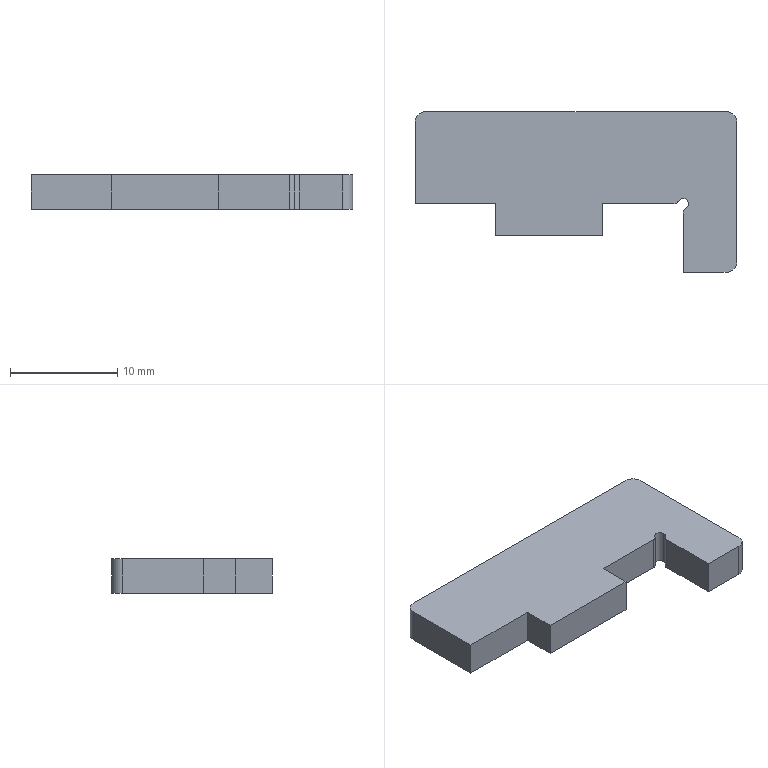Part | SolidWorks | features FlatPattern 1, SMBaseFlange 1, SheetMetal 1 | 1 solid | 19 faces | box 30 x 15 x 3.2 mm | volume 1020 mm3 | plane 12 | cylinder 7 | commonest cylinder face diameters 1 x4 2 x3
STEP:
#1=CARTESIAN_POINT('',(60.127,-203.35,-3.2));
#2=VERTEX_POINT('',#1);
#3=CARTESIAN_POINT('',(61.06,-203.6,-3.2));
#4=VERTEX_POINT('',#3);
#5=CARTESIAN_POINT('',(60.56,-203.6,-3.2));
#6=DIRECTION('',(0.,0.,-1.));
#7=DIRECTION('',(1.,0.,0.));
#8=AXIS2_PLACEMENT_3D('',#5,#6,#7);
#9=CIRCLE('',#8,0.5);
#10=EDGE_CURVE('',#2,#4,#9,.T.);
#11=ORIENTED_EDGE('',*,*,#10,.T.);
#12=CARTESIAN_POINT('',(61.06,-203.6,0.));
#13=VERTEX_POINT('',#12);
#14=CARTESIAN_POINT('',(61.06,-203.6,-3.2));
#15=DIRECTION('',(0.,0.,1.));
#16=VECTOR('',#15,1000.);
#17=LINE('',#14,#16);
#18=EDGE_CURVE('',#4,#13,#17,.T.);
#19=ORIENTED_EDGE('',*,*,#18,.T.);
#20=CARTESIAN_POINT('',(60.127,-203.35,0.));
#21=VERTEX_POINT('',#20);
#22=CARTESIAN_POINT('',(60.56,-203.6,0.));
#23=DIRECTION('',(0.,0.,-1.));
#24=DIRECTION('',(1.,0.,0.));
#25=AXIS2_PLACEMENT_3D('',#22,#23,#24);
#26=CIRCLE('',#25,0.5);
#27=EDGE_CURVE('',#21,#13,#26,.T.);
#28=ORIENTED_EDGE('',*,*,#27,.F.);
#29=CARTESIAN_POINT('',(60.127,-203.35,-3.2));
#30=DIRECTION('',(0.,0.,1.));
#31=VECTOR('',#30,1000.);
#32=LINE('',#29,#31);
#33=EDGE_CURVE('',#2,#21,#32,.T.);
#34=ORIENTED_EDGE('',*,*,#33,.F.);
#35=EDGE_LOOP('',(#11,#19,#28,#34));
#36=FACE_OUTER_BOUND('',#35,.T.);
#37=CARTESIAN_POINT('',(60.56,-203.6,-3.2));
#38=DIRECTION('',(0.,0.,1.));
#39=DIRECTION('',(1.,0.,0.));
#40=AXIS2_PLACEMENT_3D('',#37,#38,#39);
#41=CYLINDRICAL_SURFACE('',#40,0.5);
#42=ADVANCED_FACE('',(#36),#41,.F.);
#43=CARTESIAN_POINT('',(60.56,-204.466,0.));
#44=VERTEX_POINT('',#43);
#45=CARTESIAN_POINT('',(60.56,-210.,0.));
#46=VERTEX_POINT('',#45);
#47=CARTESIAN_POINT('',(60.56,-204.466,0.));
#48=DIRECTION('',(0.,-1.,0.));
#49=VECTOR('',#48,1000.);
#50=LINE('',#47,#49);
#51=EDGE_CURVE('',#44,#46,#50,.T.);
#52=ORIENTED_EDGE('',*,*,#51,.F.);
#53=CARTESIAN_POINT('',(60.56,-204.466,-3.2));
#54=VERTEX_POINT('',#53);
#55=CARTESIAN_POINT('',(60.56,-204.466,-3.2));
#56=DIRECTION('',(0.,0.,1.));
#57=VECTOR('',#56,1000.);
#58=LINE('',#55,#57);
#59=EDGE_CURVE('',#54,#44,#58,.T.);
#60=ORIENTED_EDGE('',*,*,#59,.F.);
#61=CARTESIAN_POINT('',(60.56,-210.,-3.2));
#62=VERTEX_POINT('',#61);
#63=CARTESIAN_POINT('',(60.56,-204.466,-3.2));
#64=DIRECTION('',(0.,-1.,0.));
#65=VECTOR('',#64,1000.);
#66=LINE('',#63,#65);
#67=EDGE_CURVE('',#54,#62,#66,.T.);
#68=ORIENTED_EDGE('',*,*,#67,.T.);
#69=CARTESIAN_POINT('',(60.56,-210.,-3.2));
#70=DIRECTION('',(0.,0.,1.));
#71=VECTOR('',#70,1000.);
#72=LINE('',#69,#71);
#73=EDGE_CURVE('',#62,#46,#72,.T.);
#74=ORIENTED_EDGE('',*,*,#73,.T.);
#75=EDGE_LOOP('',(#52,#60,#68,#74));
#76=FACE_OUTER_BOUND('',#75,.T.);
#77=CARTESIAN_POINT('',(60.56,-204.466,-3.2));
#78=DIRECTION('',(-1.,0.,0.));
#79=DIRECTION('',(0.,-1.,0.));
#80=AXIS2_PLACEMENT_3D('',#77,#78,#79);
#81=PLANE('',#80);
#82=ADVANCED_FACE('',(#76),#81,.T.);
#83=CARTESIAN_POINT('',(60.81,-204.033,0.));
#84=VERTEX_POINT('',#83);
#85=CARTESIAN_POINT('',(61.06,-204.466,0.));
#86=DIRECTION('',(0.,0.,1.));
#87=DIRECTION('',(1.,0.,0.));
#88=AXIS2_PLACEMENT_3D('',#85,#86,#87);
#89=CIRCLE('',#88,0.5);
#90=EDGE_CURVE('',#84,#44,#89,.T.);
#91=ORIENTED_EDGE('',*,*,#90,.F.);
#92=CARTESIAN_POINT('',(60.81,-204.033,-3.2));
#93=VERTEX_POINT('',#92);
#94=CARTESIAN_POINT('',(60.81,-204.033,-3.2));
#95=DIRECTION('',(0.,0.,1.));
#96=VECTOR('',#95,1000.);
#97=LINE('',#94,#96);
#98=EDGE_CURVE('',#93,#84,#97,.T.);
#99=ORIENTED_EDGE('',*,*,#98,.F.);
#100=CARTESIAN_POINT('',(61.06,-204.466,-3.2));
#101=DIRECTION('',(0.,0.,1.));
#102=DIRECTION('',(1.,0.,0.));
#103=AXIS2_PLACEMENT_3D('',#100,#101,#102);
#104=CIRCLE('',#103,0.5);
#105=EDGE_CURVE('',#93,#54,#104,.T.);
#106=ORIENTED_EDGE('',*,*,#105,.T.);
#107=ORIENTED_EDGE('',*,*,#59,.T.);
#108=EDGE_LOOP('',(#91,#99,#106,#107));
#109=FACE_OUTER_BOUND('',#108,.T.);
#110=CARTESIAN_POINT('',(61.06,-204.466,-3.2));
#111=DIRECTION('',(0.,0.,1.));
#112=DIRECTION('',(1.,0.,0.));
#113=AXIS2_PLACEMENT_3D('',#110,#111,#112);
#114=CYLINDRICAL_SURFACE('',#113,0.5);
#115=ADVANCED_FACE('',(#109),#114,.T.);
#116=ORIENTED_EDGE('',*,*,#18,.F.);
#117=CARTESIAN_POINT('',(60.56,-203.6,-3.2));
#118=DIRECTION('',(0.,0.,-1.));
#119=DIRECTION('',(1.,0.,0.));
#120=AXIS2_PLACEMENT_3D('',#117,#118,#119);
#121=CIRCLE('',#120,0.5);
#122=EDGE_CURVE('',#4,#93,#121,.T.);
#123=ORIENTED_EDGE('',*,*,#122,.T.);
#124=ORIENTED_EDGE('',*,*,#98,.T.);
#125=CARTESIAN_POINT('',(60.56,-203.6,0.));
#126=DIRECTION('',(0.,0.,-1.));
#127=DIRECTION('',(1.,0.,0.));
#128=AXIS2_PLACEMENT_3D('',#125,#126,#127);
#129=CIRCLE('',#128,0.5);
#130=EDGE_CURVE('',#13,#84,#129,.T.);
#131=ORIENTED_EDGE('',*,*,#130,.F.);
#132=EDGE_LOOP('',(#116,#123,#124,#131));
#133=FACE_OUTER_BOUND('',#132,.T.);
#134=CARTESIAN_POINT('',(60.56,-203.6,-3.2));
#135=DIRECTION('',(0.,0.,1.));
#136=DIRECTION('',(1.,0.,0.));
#137=AXIS2_PLACEMENT_3D('',#134,#135,#136);
#138=CYLINDRICAL_SURFACE('',#137,0.5);
#139=ADVANCED_FACE('',(#133),#138,.F.);
#140=CARTESIAN_POINT('',(59.694,-203.6,0.));
#141=VERTEX_POINT('',#140);
#142=CARTESIAN_POINT('',(59.694,-203.1,0.));
#143=DIRECTION('',(0.,0.,1.));
#144=DIRECTION('',(-1.,0.,0.));
#145=AXIS2_PLACEMENT_3D('',#142,#143,#144);
#146=CIRCLE('',#145,0.5);
#147=EDGE_CURVE('',#141,#21,#146,.T.);
#148=ORIENTED_EDGE('',*,*,#147,.F.);
#149=CARTESIAN_POINT('',(59.694,-203.6,-3.2));
#150=VERTEX_POINT('',#149);
#151=CARTESIAN_POINT('',(59.694,-203.6,-3.2));
#152=DIRECTION('',(0.,0.,1.));
#153=VECTOR('',#152,1000.);
#154=LINE('',#151,#153);
#155=EDGE_CURVE('',#150,#141,#154,.T.);
#156=ORIENTED_EDGE('',*,*,#155,.F.);
#157=CARTESIAN_POINT('',(59.694,-203.1,-3.2));
#158=DIRECTION('',(0.,0.,1.));
#159=DIRECTION('',(-1.,0.,0.));
#160=AXIS2_PLACEMENT_3D('',#157,#158,#159);
#161=CIRCLE('',#160,0.5);
#162=EDGE_CURVE('',#150,#2,#161,.T.);
#163=ORIENTED_EDGE('',*,*,#162,.T.);
#164=ORIENTED_EDGE('',*,*,#33,.T.);
#165=EDGE_LOOP('',(#148,#156,#163,#164));
#166=FACE_OUTER_BOUND('',#165,.T.);
#167=CARTESIAN_POINT('',(59.694,-203.1,-3.2));
#168=DIRECTION('',(0.,0.,1.));
#169=DIRECTION('',(1.,0.,0.));
#170=AXIS2_PLACEMENT_3D('',#167,#168,#169);
#171=CYLINDRICAL_SURFACE('',#170,0.5);
#172=ADVANCED_FACE('',(#166),#171,.T.);
#173=CARTESIAN_POINT('',(53.06,-203.6,0.));
#174=VERTEX_POINT('',#173);
#175=CARTESIAN_POINT('',(53.06,-203.6,0.));
#176=DIRECTION('',(1.,0.,0.));
#177=VECTOR('',#176,1000.);
#178=LINE('',#175,#177);
#179=EDGE_CURVE('',#174,#141,#178,.T.);
#180=ORIENTED_EDGE('',*,*,#179,.F.);
#181=CARTESIAN_POINT('',(53.06,-203.6,-3.2));
#182=VERTEX_POINT('',#181);
#183=CARTESIAN_POINT('',(53.06,-203.6,-3.2));
#184=DIRECTION('',(0.,0.,1.));
#185=VECTOR('',#184,1000.);
#186=LINE('',#183,#185);
#187=EDGE_CURVE('',#182,#174,#186,.T.);
#188=ORIENTED_EDGE('',*,*,#187,.F.);
#189=CARTESIAN_POINT('',(53.06,-203.6,-3.2));
#190=DIRECTION('',(1.,0.,0.));
#191=VECTOR('',#190,1000.);
#192=LINE('',#189,#191);
#193=EDGE_CURVE('',#182,#150,#192,.T.);
#194=ORIENTED_EDGE('',*,*,#193,.T.);
#195=ORIENTED_EDGE('',*,*,#155,.T.);
#196=EDGE_LOOP('',(#180,#188,#194,#195));
#197=FACE_OUTER_BOUND('',#196,.T.);
#198=CARTESIAN_POINT('',(53.06,-203.6,-3.2));
#199=DIRECTION('',(0.,-1.,0.));
#200=DIRECTION('',(0.,0.,-1.));
#201=AXIS2_PLACEMENT_3D('',#198,#199,#200);
#202=PLANE('',#201);
#203=ADVANCED_FACE('',(#197),#202,.T.);
#204=CARTESIAN_POINT('',(53.06,-206.6,0.));
#205=VERTEX_POINT('',#204);
#206=CARTESIAN_POINT('',(53.06,-206.6,0.));
#207=DIRECTION('',(0.,1.,0.));
#208=VECTOR('',#207,1000.);
#209=LINE('',#206,#208);
#210=EDGE_CURVE('',#205,#174,#209,.T.);
#211=ORIENTED_EDGE('',*,*,#210,.F.);
#212=CARTESIAN_POINT('',(53.06,-206.6,-3.2));
#213=VERTEX_POINT('',#212);
#214=CARTESIAN_POINT('',(53.06,-206.6,-3.2));
#215=DIRECTION('',(0.,0.,1.));
#216=VECTOR('',#215,1000.);
#217=LINE('',#214,#216);
#218=EDGE_CURVE('',#213,#205,#217,.T.);
#219=ORIENTED_EDGE('',*,*,#218,.F.);
#220=CARTESIAN_POINT('',(53.06,-206.6,-3.2));
#221=DIRECTION('',(0.,1.,0.));
#222=VECTOR('',#221,1000.);
#223=LINE('',#220,#222);
#224=EDGE_CURVE('',#213,#182,#223,.T.);
#225=ORIENTED_EDGE('',*,*,#224,.T.);
#226=ORIENTED_EDGE('',*,*,#187,.T.);
#227=EDGE_LOOP('',(#211,#219,#225,#226));
#228=FACE_OUTER_BOUND('',#227,.T.);
#229=CARTESIAN_POINT('',(53.06,-206.6,-3.2));
#230=DIRECTION('',(1.,0.,0.));
#231=DIRECTION('',(0.,0.,-1.));
#232=AXIS2_PLACEMENT_3D('',#229,#230,#231);
#233=PLANE('',#232);
#234=ADVANCED_FACE('',(#228),#233,.T.);
#235=CARTESIAN_POINT('',(43.06,-206.6,0.));
#236=VERTEX_POINT('',#235);
#237=CARTESIAN_POINT('',(43.06,-206.6,0.));
#238=DIRECTION('',(1.,0.,0.));
#239=VECTOR('',#238,1000.);
#240=LINE('',#237,#239);
#241=EDGE_CURVE('',#236,#205,#240,.T.);
#242=ORIENTED_EDGE('',*,*,#241,.F.);
#243=CARTESIAN_POINT('',(43.06,-206.6,-3.2));
#244=VERTEX_POINT('',#243);
#245=CARTESIAN_POINT('',(43.06,-206.6,-3.2));
#246=DIRECTION('',(0.,0.,1.));
#247=VECTOR('',#246,1000.);
#248=LINE('',#245,#247);
#249=EDGE_CURVE('',#244,#236,#248,.T.);
#250=ORIENTED_EDGE('',*,*,#249,.F.);
#251=CARTESIAN_POINT('',(43.06,-206.6,-3.2));
#252=DIRECTION('',(1.,0.,0.));
#253=VECTOR('',#252,1000.);
#254=LINE('',#251,#253);
#255=EDGE_CURVE('',#244,#213,#254,.T.);
#256=ORIENTED_EDGE('',*,*,#255,.T.);
#257=ORIENTED_EDGE('',*,*,#218,.T.);
#258=EDGE_LOOP('',(#242,#250,#256,#257));
#259=FACE_OUTER_BOUND('',#258,.T.);
#260=CARTESIAN_POINT('',(43.06,-206.6,-3.2));
#261=DIRECTION('',(0.,-1.,0.));
#262=DIRECTION('',(0.,0.,-1.));
#263=AXIS2_PLACEMENT_3D('',#260,#261,#262);
#264=PLANE('',#263);
#265=ADVANCED_FACE('',(#259),#264,.T.);
#266=CARTESIAN_POINT('',(43.06,-203.6,0.));
#267=VERTEX_POINT('',#266);
#268=CARTESIAN_POINT('',(43.06,-203.6,0.));
#269=DIRECTION('',(0.,-1.,0.));
#270=VECTOR('',#269,1000.);
#271=LINE('',#268,#270);
#272=EDGE_CURVE('',#267,#236,#271,.T.);
#273=ORIENTED_EDGE('',*,*,#272,.F.);
#274=CARTESIAN_POINT('',(43.06,-203.6,-3.2));
#275=VERTEX_POINT('',#274);
#276=CARTESIAN_POINT('',(43.06,-203.6,-3.2));
#277=DIRECTION('',(0.,0.,1.));
#278=VECTOR('',#277,1000.);
#279=LINE('',#276,#278);
#280=EDGE_CURVE('',#275,#267,#279,.T.);
#281=ORIENTED_EDGE('',*,*,#280,.F.);
#282=CARTESIAN_POINT('',(43.06,-203.6,-3.2));
#283=DIRECTION('',(0.,-1.,0.));
#284=VECTOR('',#283,1000.);
#285=LINE('',#282,#284);
#286=EDGE_CURVE('',#275,#244,#285,.T.);
#287=ORIENTED_EDGE('',*,*,#286,.T.);
#288=ORIENTED_EDGE('',*,*,#249,.T.);
#289=EDGE_LOOP('',(#273,#281,#287,#288));
#290=FACE_OUTER_BOUND('',#289,.T.);
#291=CARTESIAN_POINT('',(43.06,-203.6,-3.2));
#292=DIRECTION('',(-1.,0.,0.));
#293=DIRECTION('',(0.,0.,1.));
#294=AXIS2_PLACEMENT_3D('',#291,#292,#293);
#295=PLANE('',#294);
#296=ADVANCED_FACE('',(#290),#295,.T.);
#297=CARTESIAN_POINT('',(35.56,-203.6,0.));
#298=VERTEX_POINT('',#297);
#299=CARTESIAN_POINT('',(35.56,-203.6,0.));
#300=DIRECTION('',(1.,0.,0.));
#301=VECTOR('',#300,1000.);
#302=LINE('',#299,#301);
#303=EDGE_CURVE('',#298,#267,#302,.T.);
#304=ORIENTED_EDGE('',*,*,#303,.F.);
#305=CARTESIAN_POINT('',(35.56,-203.6,-3.2));
#306=VERTEX_POINT('',#305);
#307=CARTESIAN_POINT('',(35.56,-203.6,-3.2));
#308=DIRECTION('',(0.,0.,1.));
#309=VECTOR('',#308,1000.);
#310=LINE('',#307,#309);
#311=EDGE_CURVE('',#306,#298,#310,.T.);
#312=ORIENTED_EDGE('',*,*,#311,.F.);
#313=CARTESIAN_POINT('',(35.56,-203.6,-3.2));
#314=DIRECTION('',(1.,0.,0.));
#315=VECTOR('',#314,1000.);
#316=LINE('',#313,#315);
#317=EDGE_CURVE('',#306,#275,#316,.T.);
#318=ORIENTED_EDGE('',*,*,#317,.T.);
#319=ORIENTED_EDGE('',*,*,#280,.T.);
#320=EDGE_LOOP('',(#304,#312,#318,#319));
#321=FACE_OUTER_BOUND('',#320,.T.);
#322=CARTESIAN_POINT('',(35.56,-203.6,-3.2));
#323=DIRECTION('',(0.,-1.,0.));
#324=DIRECTION('',(0.,0.,-1.));
#325=AXIS2_PLACEMENT_3D('',#322,#323,#324);
#326=PLANE('',#325);
#327=ADVANCED_FACE('',(#321),#326,.T.);
#328=CARTESIAN_POINT('',(35.56,-196.,0.));
#329=VERTEX_POINT('',#328);
#330=CARTESIAN_POINT('',(35.56,-196.,0.));
#331=DIRECTION('',(0.,-1.,0.));
#332=VECTOR('',#331,1000.);
#333=LINE('',#330,#332);
#334=EDGE_CURVE('',#329,#298,#333,.T.);
#335=ORIENTED_EDGE('',*,*,#334,.F.);
#336=CARTESIAN_POINT('',(35.56,-196.,-3.2));
#337=VERTEX_POINT('',#336);
#338=CARTESIAN_POINT('',(35.56,-196.,-3.2));
#339=DIRECTION('',(0.,0.,1.));
#340=VECTOR('',#339,1000.);
#341=LINE('',#338,#340);
#342=EDGE_CURVE('',#337,#329,#341,.T.);
#343=ORIENTED_EDGE('',*,*,#342,.F.);
#344=CARTESIAN_POINT('',(35.56,-196.,-3.2));
#345=DIRECTION('',(0.,-1.,0.));
#346=VECTOR('',#345,1000.);
#347=LINE('',#344,#346);
#348=EDGE_CURVE('',#337,#306,#347,.T.);
#349=ORIENTED_EDGE('',*,*,#348,.T.);
#350=ORIENTED_EDGE('',*,*,#311,.T.);
#351=EDGE_LOOP('',(#335,#343,#349,#350));
#352=FACE_OUTER_BOUND('',#351,.T.);
#353=CARTESIAN_POINT('',(35.56,-196.,-3.2));
#354=DIRECTION('',(-1.,0.,0.));
#355=DIRECTION('',(0.,0.,1.));
#356=AXIS2_PLACEMENT_3D('',#353,#354,#355);
#357=PLANE('',#356);
#358=ADVANCED_FACE('',(#352),#357,.T.);
#359=CARTESIAN_POINT('',(36.56,-195.,0.));
#360=VERTEX_POINT('',#359);
#361=CARTESIAN_POINT('',(36.56,-196.,0.));
#362=DIRECTION('',(0.,0.,1.));
#363=DIRECTION('',(1.,0.,0.));
#364=AXIS2_PLACEMENT_3D('',#361,#362,#363);
#365=CIRCLE('',#364,1.);
#366=EDGE_CURVE('',#360,#329,#365,.T.);
#367=ORIENTED_EDGE('',*,*,#366,.F.);
#368=CARTESIAN_POINT('',(36.56,-195.,-3.2));
#369=VERTEX_POINT('',#368);
#370=CARTESIAN_POINT('',(36.56,-195.,-3.2));
#371=DIRECTION('',(0.,0.,1.));
#372=VECTOR('',#371,1000.);
#373=LINE('',#370,#372);
#374=EDGE_CURVE('',#369,#360,#373,.T.);
#375=ORIENTED_EDGE('',*,*,#374,.F.);
#376=CARTESIAN_POINT('',(36.56,-196.,-3.2));
#377=DIRECTION('',(0.,0.,1.));
#378=DIRECTION('',(1.,0.,0.));
#379=AXIS2_PLACEMENT_3D('',#376,#377,#378);
#380=CIRCLE('',#379,1.);
#381=EDGE_CURVE('',#369,#337,#380,.T.);
#382=ORIENTED_EDGE('',*,*,#381,.T.);
#383=ORIENTED_EDGE('',*,*,#342,.T.);
#384=EDGE_LOOP('',(#367,#375,#382,#383));
#385=FACE_OUTER_BOUND('',#384,.T.);
#386=CARTESIAN_POINT('',(36.56,-196.,-3.2));
#387=DIRECTION('',(0.,0.,1.));
#388=DIRECTION('',(1.,0.,0.));
#389=AXIS2_PLACEMENT_3D('',#386,#387,#388);
#390=CYLINDRICAL_SURFACE('',#389,1.);
#391=ADVANCED_FACE('',(#385),#390,.T.);
#392=CARTESIAN_POINT('',(64.56,-195.,0.));
#393=VERTEX_POINT('',#392);
#394=CARTESIAN_POINT('',(64.56,-195.,0.));
#395=DIRECTION('',(-1.,0.,0.));
#396=VECTOR('',#395,1000.);
#397=LINE('',#394,#396);
#398=EDGE_CURVE('',#393,#360,#397,.T.);
#399=ORIENTED_EDGE('',*,*,#398,.F.);
#400=CARTESIAN_POINT('',(64.56,-195.,-3.2));
#401=VERTEX_POINT('',#400);
#402=CARTESIAN_POINT('',(64.56,-195.,-3.2));
#403=DIRECTION('',(0.,0.,1.));
#404=VECTOR('',#403,1000.);
#405=LINE('',#402,#404);
#406=EDGE_CURVE('',#401,#393,#405,.T.);
#407=ORIENTED_EDGE('',*,*,#406,.F.);
#408=CARTESIAN_POINT('',(64.56,-195.,-3.2));
#409=DIRECTION('',(-1.,0.,0.));
#410=VECTOR('',#409,1000.);
#411=LINE('',#408,#410);
#412=EDGE_CURVE('',#401,#369,#411,.T.);
#413=ORIENTED_EDGE('',*,*,#412,.T.);
#414=ORIENTED_EDGE('',*,*,#374,.T.);
#415=EDGE_LOOP('',(#399,#407,#413,#414));
#416=FACE_OUTER_BOUND('',#415,.T.);
#417=CARTESIAN_POINT('',(64.56,-195.,-3.2));
#418=DIRECTION('',(0.,1.,0.));
#419=DIRECTION('',(0.,0.,1.));
#420=AXIS2_PLACEMENT_3D('',#417,#418,#419);
#421=PLANE('',#420);
#422=ADVANCED_FACE('',(#416),#421,.T.);
#423=CARTESIAN_POINT('',(65.56,-196.,0.));
#424=VERTEX_POINT('',#423);
#425=CARTESIAN_POINT('',(64.56,-196.,0.));
#426=DIRECTION('',(0.,0.,1.));
#427=DIRECTION('',(1.,0.,0.));
#428=AXIS2_PLACEMENT_3D('',#425,#426,#427);
#429=CIRCLE('',#428,1.);
#430=EDGE_CURVE('',#424,#393,#429,.T.);
#431=ORIENTED_EDGE('',*,*,#430,.F.);
#432=CARTESIAN_POINT('',(65.56,-196.,-3.2));
#433=VERTEX_POINT('',#432);
#434=CARTESIAN_POINT('',(65.56,-196.,-3.2));
#435=DIRECTION('',(0.,0.,1.));
#436=VECTOR('',#435,1000.);
#437=LINE('',#434,#436);
#438=EDGE_CURVE('',#433,#424,#437,.T.);
#439=ORIENTED_EDGE('',*,*,#438,.F.);
#440=CARTESIAN_POINT('',(64.56,-196.,-3.2));
#441=DIRECTION('',(0.,0.,1.));
#442=DIRECTION('',(1.,0.,0.));
#443=AXIS2_PLACEMENT_3D('',#440,#441,#442);
#444=CIRCLE('',#443,1.);
#445=EDGE_CURVE('',#433,#401,#444,.T.);
#446=ORIENTED_EDGE('',*,*,#445,.T.);
#447=ORIENTED_EDGE('',*,*,#406,.T.);
#448=EDGE_LOOP('',(#431,#439,#446,#447));
#449=FACE_OUTER_BOUND('',#448,.T.);
#450=CARTESIAN_POINT('',(64.56,-196.,-3.2));
#451=DIRECTION('',(0.,0.,1.));
#452=DIRECTION('',(1.,0.,0.));
#453=AXIS2_PLACEMENT_3D('',#450,#451,#452);
#454=CYLINDRICAL_SURFACE('',#453,1.);
#455=ADVANCED_FACE('',(#449),#454,.T.);
#456=CARTESIAN_POINT('',(65.56,-209.,0.));
#457=VERTEX_POINT('',#456);
#458=CARTESIAN_POINT('',(65.56,-209.,0.));
#459=DIRECTION('',(0.,1.,0.));
#460=VECTOR('',#459,1000.);
#461=LINE('',#458,#460);
#462=EDGE_CURVE('',#457,#424,#461,.T.);
#463=ORIENTED_EDGE('',*,*,#462,.F.);
#464=CARTESIAN_POINT('',(65.56,-209.,-3.2));
#465=VERTEX_POINT('',#464);
#466=CARTESIAN_POINT('',(65.56,-209.,-3.2));
#467=DIRECTION('',(0.,0.,1.));
#468=VECTOR('',#467,1000.);
#469=LINE('',#466,#468);
#470=EDGE_CURVE('',#465,#457,#469,.T.);
#471=ORIENTED_EDGE('',*,*,#470,.F.);
#472=CARTESIAN_POINT('',(65.56,-209.,-3.2));
#473=DIRECTION('',(0.,1.,0.));
#474=VECTOR('',#473,1000.);
#475=LINE('',#472,#474);
#476=EDGE_CURVE('',#465,#433,#475,.T.);
#477=ORIENTED_EDGE('',*,*,#476,.T.);
#478=ORIENTED_EDGE('',*,*,#438,.T.);
#479=EDGE_LOOP('',(#463,#471,#477,#478));
#480=FACE_OUTER_BOUND('',#479,.T.);
#481=CARTESIAN_POINT('',(65.56,-209.,-3.2));
#482=DIRECTION('',(1.,0.,0.));
#483=DIRECTION('',(0.,0.,-1.));
#484=AXIS2_PLACEMENT_3D('',#481,#482,#483);
#485=PLANE('',#484);
#486=ADVANCED_FACE('',(#480),#485,.T.);
#487=CARTESIAN_POINT('',(64.56,-210.,0.));
#488=VERTEX_POINT('',#487);
#489=CARTESIAN_POINT('',(64.56,-209.,0.));
#490=DIRECTION('',(0.,0.,1.));
#491=DIRECTION('',(1.,0.,0.));
#492=AXIS2_PLACEMENT_3D('',#489,#490,#491);
#493=CIRCLE('',#492,1.);
#494=EDGE_CURVE('',#488,#457,#493,.T.);
#495=ORIENTED_EDGE('',*,*,#494,.F.);
#496=CARTESIAN_POINT('',(64.56,-210.,-3.2));
#497=VERTEX_POINT('',#496);
#498=CARTESIAN_POINT('',(64.56,-210.,-3.2));
#499=DIRECTION('',(0.,0.,1.));
#500=VECTOR('',#499,1000.);
#501=LINE('',#498,#500);
#502=EDGE_CURVE('',#497,#488,#501,.T.);
#503=ORIENTED_EDGE('',*,*,#502,.F.);
#504=CARTESIAN_POINT('',(64.56,-209.,-3.2));
#505=DIRECTION('',(0.,0.,1.));
#506=DIRECTION('',(1.,0.,0.));
#507=AXIS2_PLACEMENT_3D('',#504,#505,#506);
#508=CIRCLE('',#507,1.);
#509=EDGE_CURVE('',#497,#465,#508,.T.);
#510=ORIENTED_EDGE('',*,*,#509,.T.);
#511=ORIENTED_EDGE('',*,*,#470,.T.);
#512=EDGE_LOOP('',(#495,#503,#510,#511));
#513=FACE_OUTER_BOUND('',#512,.T.);
#514=CARTESIAN_POINT('',(64.56,-209.,-3.2));
#515=DIRECTION('',(0.,0.,1.));
#516=DIRECTION('',(1.,0.,0.));
#517=AXIS2_PLACEMENT_3D('',#514,#515,#516);
#518=CYLINDRICAL_SURFACE('',#517,1.);
#519=ADVANCED_FACE('',(#513),#518,.T.);
#520=CARTESIAN_POINT('',(60.56,-210.,0.));
#521=DIRECTION('',(1.,0.,0.));
#522=VECTOR('',#521,1000.);
#523=LINE('',#520,#522);
#524=EDGE_CURVE('',#46,#488,#523,.T.);
#525=ORIENTED_EDGE('',*,*,#524,.F.);
#526=ORIENTED_EDGE('',*,*,#73,.F.);
#527=CARTESIAN_POINT('',(60.56,-210.,-3.2));
#528=DIRECTION('',(1.,0.,0.));
#529=VECTOR('',#528,1000.);
#530=LINE('',#527,#529);
#531=EDGE_CURVE('',#62,#497,#530,.T.);
#532=ORIENTED_EDGE('',*,*,#531,.T.);
#533=ORIENTED_EDGE('',*,*,#502,.T.);
#534=EDGE_LOOP('',(#525,#526,#532,#533));
#535=FACE_OUTER_BOUND('',#534,.T.);
#536=CARTESIAN_POINT('',(60.56,-210.,-3.2));
#537=DIRECTION('',(0.,-1.,0.));
#538=DIRECTION('',(0.,0.,-1.));
#539=AXIS2_PLACEMENT_3D('',#536,#537,#538);
#540=PLANE('',#539);
#541=ADVANCED_FACE('',(#535),#540,.T.);
#542=ORIENTED_EDGE('',*,*,#67,.F.);
#543=ORIENTED_EDGE('',*,*,#105,.F.);
#544=ORIENTED_EDGE('',*,*,#122,.F.);
#545=ORIENTED_EDGE('',*,*,#10,.F.);
#546=ORIENTED_EDGE('',*,*,#162,.F.);
#547=ORIENTED_EDGE('',*,*,#193,.F.);
#548=ORIENTED_EDGE('',*,*,#224,.F.);
#549=ORIENTED_EDGE('',*,*,#255,.F.);
#550=ORIENTED_EDGE('',*,*,#286,.F.);
#551=ORIENTED_EDGE('',*,*,#317,.F.);
#552=ORIENTED_EDGE('',*,*,#348,.F.);
#553=ORIENTED_EDGE('',*,*,#381,.F.);
#554=ORIENTED_EDGE('',*,*,#412,.F.);
#555=ORIENTED_EDGE('',*,*,#445,.F.);
#556=ORIENTED_EDGE('',*,*,#476,.F.);
#557=ORIENTED_EDGE('',*,*,#509,.F.);
#558=ORIENTED_EDGE('',*,*,#531,.F.);
#559=EDGE_LOOP('',(#542,#543,#544,#545,#546,#547,#548,#549,#550,#551,#552,#553,#554,#555,#556,#557,#558));
#560=FACE_OUTER_BOUND('',#559,.T.);
#561=CARTESIAN_POINT('',(64.56,-209.,-3.2));
#562=DIRECTION('',(0.,0.,1.));
#563=DIRECTION('',(1.,0.,0.));
#564=AXIS2_PLACEMENT_3D('',#561,#562,#563);
#565=PLANE('',#564);
#566=ADVANCED_FACE('',(#560),#565,.F.);
#567=ORIENTED_EDGE('',*,*,#51,.T.);
#568=ORIENTED_EDGE('',*,*,#524,.T.);
#569=ORIENTED_EDGE('',*,*,#494,.T.);
#570=ORIENTED_EDGE('',*,*,#462,.T.);
#571=ORIENTED_EDGE('',*,*,#430,.T.);
#572=ORIENTED_EDGE('',*,*,#398,.T.);
#573=ORIENTED_EDGE('',*,*,#366,.T.);
#574=ORIENTED_EDGE('',*,*,#334,.T.);
#575=ORIENTED_EDGE('',*,*,#303,.T.);
#576=ORIENTED_EDGE('',*,*,#272,.T.);
#577=ORIENTED_EDGE('',*,*,#241,.T.);
#578=ORIENTED_EDGE('',*,*,#210,.T.);
#579=ORIENTED_EDGE('',*,*,#179,.T.);
#580=ORIENTED_EDGE('',*,*,#147,.T.);
#581=ORIENTED_EDGE('',*,*,#27,.T.);
#582=ORIENTED_EDGE('',*,*,#130,.T.);
#583=ORIENTED_EDGE('',*,*,#90,.T.);
#584=EDGE_LOOP('',(#567,#568,#569,#570,#571,#572,#573,#574,#575,#576,#577,#578,#579,#580,#581,#582,#583));
#585=FACE_OUTER_BOUND('',#584,.T.);
#586=CARTESIAN_POINT('',(64.56,-209.,0.));
#587=DIRECTION('',(0.,0.,1.));
#588=DIRECTION('',(1.,0.,0.));
#589=AXIS2_PLACEMENT_3D('',#586,#587,#588);
#590=PLANE('',#589);
#591=ADVANCED_FACE('',(#585),#590,.T.);
#592=CLOSED_SHELL('',(#42,#82,#115,#139,#172,#203,#234,#265,#296,#327,#358,#391,#422,#455,#486,#519,#541,#566,#591));
#593=MANIFOLD_SOLID_BREP('',#592);
#594=CARTESIAN_POINT('',(0.,0.,0.));
#595=DIRECTION('',(0.,0.,1.));
#596=DIRECTION('',(1.,0.,0.));
#597=AXIS2_PLACEMENT_3D('',#594,#595,#596);
#598=(LENGTH_UNIT()NAMED_UNIT(*)SI_UNIT(.MILLI.,.METRE.));
#599=UNCERTAINTY_MEASURE_WITH_UNIT(LENGTH_MEASURE(0.00001),#598,'','');
#600=(NAMED_UNIT(*)PLANE_ANGLE_UNIT()SI_UNIT($,.RADIAN.));
#601=(NAMED_UNIT(*)SI_UNIT($,.STERADIAN.)SOLID_ANGLE_UNIT());
#602=(GEOMETRIC_REPRESENTATION_CONTEXT(3)GLOBAL_UNCERTAINTY_ASSIGNED_CONTEXT((#599))GLOBAL_UNIT_ASSIGNED_CONTEXT((#598,#600,#601))REPRESENTATION_CONTEXT('',''));
#603=ADVANCED_BREP_SHAPE_REPRESENTATION('',(#593,#597),#602);